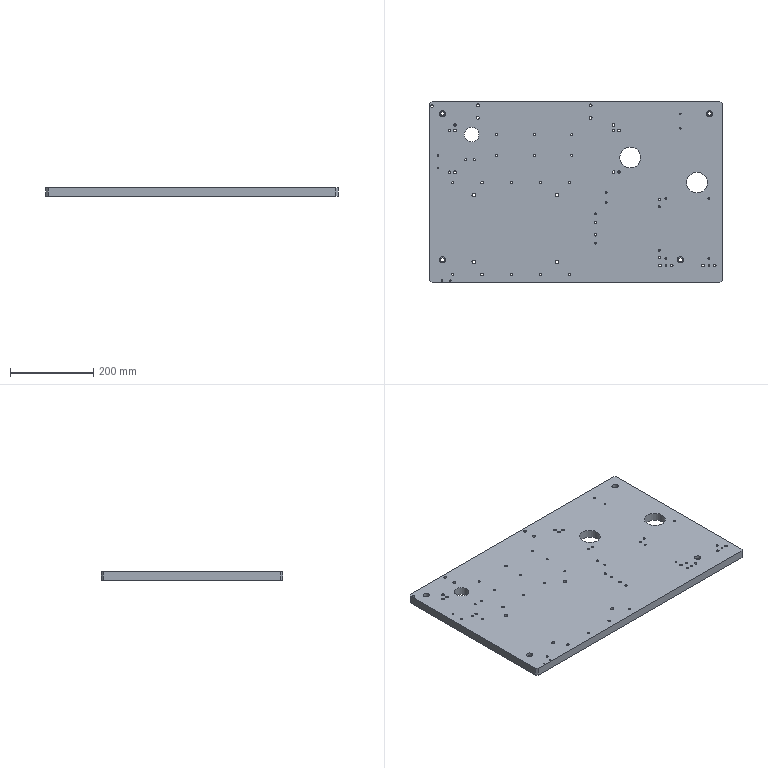Part | 1 solid | 98 faces | box 700 x 435 x 20 mm | volume 5950913 mm3 | cylinder 74 | plane 14 | cone 10 | commonest cylinder face diameters 6 x21 5 x20 6.8 x8 3.3 x6 4.2 x4 8.5 x4